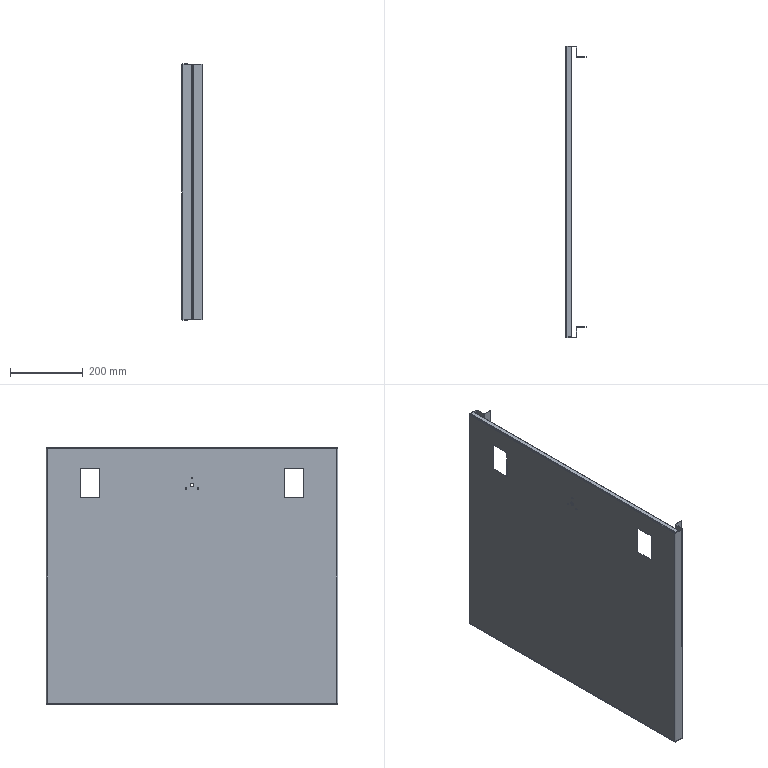Part | STEP file | SOLID | 1 solid | 82 faces | box 55 x 800 x 705 mm | volume 825706 mm3 | plane 46 | cylinder 20 | spline 16 | commonest cylinder face diameters 3 x8 5.4 x8 4.5 x3 10 x1